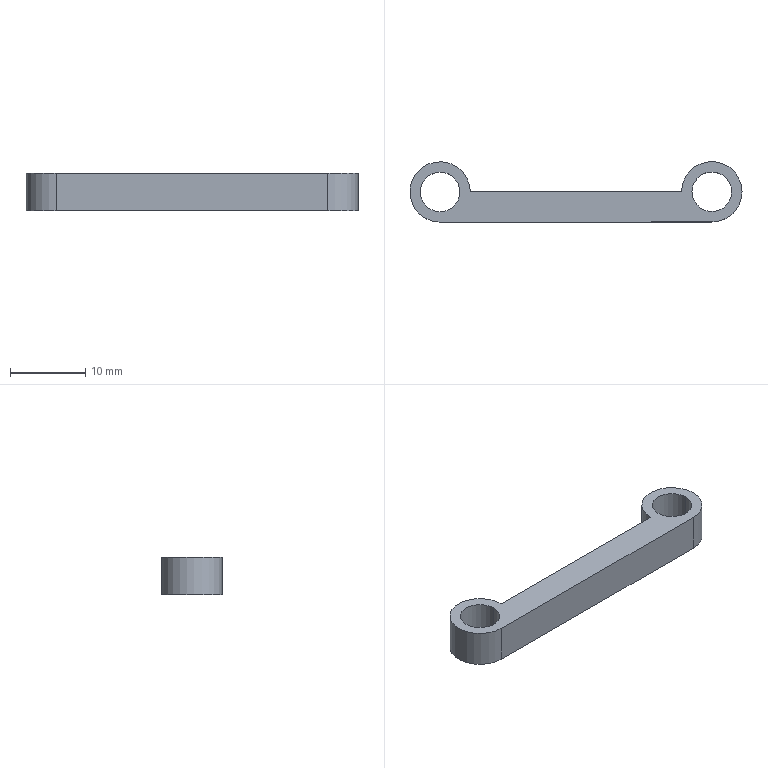Part | SolidWorks | features ICE 10, Fillet 4, Attribute 1, Extrusion 1 | 1 solid | 11 faces | box 44 x 8.023 x 5 mm | volume 880.516 mm3 | cylinder 7 | plane 4 | commonest cylinder face diameters 5.25 x4 8 x3
STEP:
#1=CARTESIAN_POINT('',(-13.375,0.,0.));
#2=VERTEX_POINT('',#1);
#3=CARTESIAN_POINT('',(-18.625,0.,0.));
#4=VERTEX_POINT('',#3);
#5=CARTESIAN_POINT('',(-16.,0.,0.));
#6=DIRECTION('',(0.,0.,-1.));
#7=DIRECTION('',(-1.,0.,0.));
#8=AXIS2_PLACEMENT_3D('',#5,#6,#7);
#9=CIRCLE('',#8,2.625);
#10=EDGE_CURVE('',#2,#4,#9,.T.);
#11=ORIENTED_EDGE('',*,*,#10,.T.);
#12=CARTESIAN_POINT('',(-18.625,0.,5.));
#13=VERTEX_POINT('',#12);
#14=CARTESIAN_POINT('',(-18.625,0.,-20.));
#15=DIRECTION('',(0.,0.,1.));
#16=VECTOR('',#15,1000.);
#17=LINE('',#14,#16);
#18=EDGE_CURVE('',#4,#13,#17,.T.);
#19=ORIENTED_EDGE('',*,*,#18,.T.);
#20=CARTESIAN_POINT('',(-13.375,0.,5.));
#21=VERTEX_POINT('',#20);
#22=CARTESIAN_POINT('',(-16.,0.,5.));
#23=DIRECTION('',(0.,0.,-1.));
#24=DIRECTION('',(-1.,0.,0.));
#25=AXIS2_PLACEMENT_3D('',#22,#23,#24);
#26=CIRCLE('',#25,2.625);
#27=EDGE_CURVE('',#21,#13,#26,.T.);
#28=ORIENTED_EDGE('',*,*,#27,.F.);
#29=CARTESIAN_POINT('',(-13.375,0.,-20.));
#30=DIRECTION('',(0.,0.,1.));
#31=VECTOR('',#30,1000.);
#32=LINE('',#29,#31);
#33=EDGE_CURVE('',#2,#21,#32,.T.);
#34=ORIENTED_EDGE('',*,*,#33,.F.);
#35=EDGE_LOOP('',(#11,#19,#28,#34));
#36=FACE_OUTER_BOUND('',#35,.T.);
#37=CARTESIAN_POINT('',(-16.,0.,-20.));
#38=DIRECTION('',(0.,0.,1.));
#39=DIRECTION('',(1.,0.,0.));
#40=AXIS2_PLACEMENT_3D('',#37,#38,#39);
#41=CYLINDRICAL_SURFACE('',#40,2.625);
#42=ADVANCED_FACE('',(#36),#41,.F.);
#43=CARTESIAN_POINT('',(17.375,0.02311,0.));
#44=VERTEX_POINT('',#43);
#45=CARTESIAN_POINT('',(22.625,0.02311,0.));
#46=VERTEX_POINT('',#45);
#47=CARTESIAN_POINT('',(20.,0.02311,0.));
#48=DIRECTION('',(0.,0.,1.));
#49=DIRECTION('',(1.,0.,0.));
#50=AXIS2_PLACEMENT_3D('',#47,#48,#49);
#51=CIRCLE('',#50,2.625);
#52=EDGE_CURVE('',#44,#46,#51,.T.);
#53=ORIENTED_EDGE('',*,*,#52,.F.);
#54=CARTESIAN_POINT('',(17.375,0.02311,5.));
#55=VERTEX_POINT('',#54);
#56=CARTESIAN_POINT('',(17.375,0.02311,0.));
#57=DIRECTION('',(0.,0.,1.));
#58=VECTOR('',#57,1000.);
#59=LINE('',#56,#58);
#60=EDGE_CURVE('',#44,#55,#59,.T.);
#61=ORIENTED_EDGE('',*,*,#60,.T.);
#62=CARTESIAN_POINT('',(22.625,0.02311,5.));
#63=VERTEX_POINT('',#62);
#64=CARTESIAN_POINT('',(20.,0.02311,5.));
#65=DIRECTION('',(0.,0.,1.));
#66=DIRECTION('',(1.,0.,0.));
#67=AXIS2_PLACEMENT_3D('',#64,#65,#66);
#68=CIRCLE('',#67,2.625);
#69=EDGE_CURVE('',#55,#63,#68,.T.);
#70=ORIENTED_EDGE('',*,*,#69,.T.);
#71=CARTESIAN_POINT('',(22.625,0.02311,0.));
#72=DIRECTION('',(0.,0.,1.));
#73=VECTOR('',#72,1000.);
#74=LINE('',#71,#73);
#75=EDGE_CURVE('',#46,#63,#74,.T.);
#76=ORIENTED_EDGE('',*,*,#75,.F.);
#77=EDGE_LOOP('',(#53,#61,#70,#76));
#78=FACE_OUTER_BOUND('',#77,.T.);
#79=CARTESIAN_POINT('',(20.,0.02311,0.));
#80=DIRECTION('',(0.,0.,1.));
#81=DIRECTION('',(1.,0.,0.));
#82=AXIS2_PLACEMENT_3D('',#79,#80,#81);
#83=CYLINDRICAL_SURFACE('',#82,2.625);
#84=ADVANCED_FACE('',(#78),#83,.F.);
#85=CARTESIAN_POINT('',(20.,-3.977,0.));
#86=VERTEX_POINT('',#85);
#87=CARTESIAN_POINT('',(24.,0.02311,0.));
#88=VERTEX_POINT('',#87);
#89=CARTESIAN_POINT('',(20.,0.02311,0.));
#90=DIRECTION('',(0.,0.,1.));
#91=DIRECTION('',(1.,0.,0.));
#92=AXIS2_PLACEMENT_3D('',#89,#90,#91);
#93=CIRCLE('',#92,4.);
#94=EDGE_CURVE('',#86,#88,#93,.T.);
#95=ORIENTED_EDGE('',*,*,#94,.T.);
#96=CARTESIAN_POINT('',(24.,0.02311,5.));
#97=VERTEX_POINT('',#96);
#98=CARTESIAN_POINT('',(24.,0.02311,0.));
#99=DIRECTION('',(0.,0.,1.));
#100=VECTOR('',#99,1000.);
#101=LINE('',#98,#100);
#102=EDGE_CURVE('',#88,#97,#101,.T.);
#103=ORIENTED_EDGE('',*,*,#102,.T.);
#104=CARTESIAN_POINT('',(20.,-3.977,5.));
#105=VERTEX_POINT('',#104);
#106=CARTESIAN_POINT('',(20.,0.02311,5.));
#107=DIRECTION('',(0.,0.,1.));
#108=DIRECTION('',(1.,0.,0.));
#109=AXIS2_PLACEMENT_3D('',#106,#107,#108);
#110=CIRCLE('',#109,4.);
#111=EDGE_CURVE('',#105,#97,#110,.T.);
#112=ORIENTED_EDGE('',*,*,#111,.F.);
#113=CARTESIAN_POINT('',(20.,-3.977,0.));
#114=DIRECTION('',(0.,0.,1.));
#115=VECTOR('',#114,1000.);
#116=LINE('',#113,#115);
#117=EDGE_CURVE('',#86,#105,#116,.T.);
#118=ORIENTED_EDGE('',*,*,#117,.F.);
#119=EDGE_LOOP('',(#95,#103,#112,#118));
#120=FACE_OUTER_BOUND('',#119,.T.);
#121=CARTESIAN_POINT('',(20.,0.02311,0.));
#122=DIRECTION('',(0.,0.,1.));
#123=DIRECTION('',(1.,0.,0.));
#124=AXIS2_PLACEMENT_3D('',#121,#122,#123);
#125=CYLINDRICAL_SURFACE('',#124,4.);
#126=ADVANCED_FACE('',(#120),#125,.T.);
#127=ORIENTED_EDGE('',*,*,#27,.T.);
#128=CARTESIAN_POINT('',(-16.,0.,5.));
#129=DIRECTION('',(0.,0.,-1.));
#130=DIRECTION('',(-1.,0.,0.));
#131=AXIS2_PLACEMENT_3D('',#128,#129,#130);
#132=CIRCLE('',#131,2.625);
#133=EDGE_CURVE('',#13,#21,#132,.T.);
#134=ORIENTED_EDGE('',*,*,#133,.T.);
#135=EDGE_LOOP('',(#127,#134));
#136=FACE_BOUND('',#135,.T.);
#137=CARTESIAN_POINT('',(-12.,0.,5.));
#138=VERTEX_POINT('',#137);
#139=CARTESIAN_POINT('',(-15.997,-4.,5.));
#140=VERTEX_POINT('',#139);
#141=CARTESIAN_POINT('',(-16.,0.,5.));
#142=DIRECTION('',(0.,0.,1.));
#143=DIRECTION('',(1.,0.,0.));
#144=AXIS2_PLACEMENT_3D('',#141,#142,#143);
#145=CIRCLE('',#144,4.);
#146=EDGE_CURVE('',#138,#140,#145,.T.);
#147=ORIENTED_EDGE('',*,*,#146,.T.);
#148=CARTESIAN_POINT('',(-16.,-4.,5.));
#149=DIRECTION('',(1.,0.0006418,0.));
#150=VECTOR('',#149,1000.);
#151=LINE('',#148,#150);
#152=EDGE_CURVE('',#140,#105,#151,.T.);
#153=ORIENTED_EDGE('',*,*,#152,.T.);
#154=ORIENTED_EDGE('',*,*,#111,.T.);
#155=CARTESIAN_POINT('',(16.,0.02311,5.));
#156=VERTEX_POINT('',#155);
#157=CARTESIAN_POINT('',(20.,0.02311,5.));
#158=DIRECTION('',(0.,0.,1.));
#159=DIRECTION('',(1.,0.,0.));
#160=AXIS2_PLACEMENT_3D('',#157,#158,#159);
#161=CIRCLE('',#160,4.);
#162=EDGE_CURVE('',#97,#156,#161,.T.);
#163=ORIENTED_EDGE('',*,*,#162,.T.);
#164=CARTESIAN_POINT('',(-12.,0.,5.));
#165=DIRECTION('',(1.,0.0008252,0.));
#166=VECTOR('',#165,1000.);
#167=LINE('',#164,#166);
#168=EDGE_CURVE('',#138,#156,#167,.T.);
#169=ORIENTED_EDGE('',*,*,#168,.F.);
#170=EDGE_LOOP('',(#147,#153,#154,#163,#169));
#171=FACE_OUTER_BOUND('',#170,.T.);
#172=CARTESIAN_POINT('',(20.,0.02311,5.));
#173=DIRECTION('',(0.,0.,1.));
#174=DIRECTION('',(1.,0.,0.));
#175=AXIS2_PLACEMENT_3D('',#172,#173,#174);
#176=CIRCLE('',#175,2.625);
#177=EDGE_CURVE('',#63,#55,#176,.T.);
#178=ORIENTED_EDGE('',*,*,#177,.F.);
#179=ORIENTED_EDGE('',*,*,#69,.F.);
#180=EDGE_LOOP('',(#178,#179));
#181=FACE_BOUND('',#180,.T.);
#182=CARTESIAN_POINT('',(0.,0.,5.));
#183=DIRECTION('',(0.,0.,-1.));
#184=DIRECTION('',(-1.,0.,0.));
#185=AXIS2_PLACEMENT_3D('',#182,#183,#184);
#186=PLANE('',#185);
#187=ADVANCED_FACE('',(#136,#171,#181),#186,.F.);
#188=CARTESIAN_POINT('',(-15.997,-4.,0.));
#189=VERTEX_POINT('',#188);
#190=CARTESIAN_POINT('',(-16.,-4.,0.));
#191=DIRECTION('',(1.,0.0006418,0.));
#192=VECTOR('',#191,1000.);
#193=LINE('',#190,#192);
#194=EDGE_CURVE('',#189,#86,#193,.T.);
#195=ORIENTED_EDGE('',*,*,#194,.F.);
#196=CARTESIAN_POINT('',(-12.,0.,0.));
#197=VERTEX_POINT('',#196);
#198=CARTESIAN_POINT('',(-16.,0.,0.));
#199=DIRECTION('',(0.,0.,1.));
#200=DIRECTION('',(1.,0.,0.));
#201=AXIS2_PLACEMENT_3D('',#198,#199,#200);
#202=CIRCLE('',#201,4.);
#203=EDGE_CURVE('',#197,#189,#202,.T.);
#204=ORIENTED_EDGE('',*,*,#203,.F.);
#205=CARTESIAN_POINT('',(16.,0.02311,0.));
#206=VERTEX_POINT('',#205);
#207=CARTESIAN_POINT('',(-12.,0.,0.));
#208=DIRECTION('',(1.,0.0008252,0.));
#209=VECTOR('',#208,1000.);
#210=LINE('',#207,#209);
#211=EDGE_CURVE('',#197,#206,#210,.T.);
#212=ORIENTED_EDGE('',*,*,#211,.T.);
#213=CARTESIAN_POINT('',(20.,0.02311,0.));
#214=DIRECTION('',(0.,0.,1.));
#215=DIRECTION('',(1.,0.,0.));
#216=AXIS2_PLACEMENT_3D('',#213,#214,#215);
#217=CIRCLE('',#216,4.);
#218=EDGE_CURVE('',#88,#206,#217,.T.);
#219=ORIENTED_EDGE('',*,*,#218,.F.);
#220=ORIENTED_EDGE('',*,*,#94,.F.);
#221=EDGE_LOOP('',(#195,#204,#212,#219,#220));
#222=FACE_OUTER_BOUND('',#221,.T.);
#223=ORIENTED_EDGE('',*,*,#10,.F.);
#224=CARTESIAN_POINT('',(-16.,0.,0.));
#225=DIRECTION('',(0.,0.,-1.));
#226=DIRECTION('',(-1.,0.,0.));
#227=AXIS2_PLACEMENT_3D('',#224,#225,#226);
#228=CIRCLE('',#227,2.625);
#229=EDGE_CURVE('',#4,#2,#228,.T.);
#230=ORIENTED_EDGE('',*,*,#229,.F.);
#231=EDGE_LOOP('',(#223,#230));
#232=FACE_BOUND('',#231,.T.);
#233=CARTESIAN_POINT('',(20.,0.02311,0.));
#234=DIRECTION('',(0.,0.,1.));
#235=DIRECTION('',(1.,0.,0.));
#236=AXIS2_PLACEMENT_3D('',#233,#234,#235);
#237=CIRCLE('',#236,2.625);
#238=EDGE_CURVE('',#46,#44,#237,.T.);
#239=ORIENTED_EDGE('',*,*,#238,.T.);
#240=ORIENTED_EDGE('',*,*,#52,.T.);
#241=EDGE_LOOP('',(#239,#240));
#242=FACE_BOUND('',#241,.T.);
#243=CARTESIAN_POINT('',(0.,0.,0.));
#244=DIRECTION('',(0.,0.,-1.));
#245=DIRECTION('',(-1.,0.,0.));
#246=AXIS2_PLACEMENT_3D('',#243,#244,#245);
#247=PLANE('',#246);
#248=ADVANCED_FACE('',(#222,#232,#242),#247,.T.);
#249=ORIENTED_EDGE('',*,*,#102,.F.);
#250=ORIENTED_EDGE('',*,*,#218,.T.);
#251=CARTESIAN_POINT('',(16.,0.02311,0.));
#252=DIRECTION('',(0.,0.,1.));
#253=VECTOR('',#252,1000.);
#254=LINE('',#251,#253);
#255=EDGE_CURVE('',#206,#156,#254,.T.);
#256=ORIENTED_EDGE('',*,*,#255,.T.);
#257=ORIENTED_EDGE('',*,*,#162,.F.);
#258=EDGE_LOOP('',(#249,#250,#256,#257));
#259=FACE_OUTER_BOUND('',#258,.T.);
#260=CARTESIAN_POINT('',(20.,0.02311,0.));
#261=DIRECTION('',(0.,0.,1.));
#262=DIRECTION('',(1.,0.,0.));
#263=AXIS2_PLACEMENT_3D('',#260,#261,#262);
#264=CYLINDRICAL_SURFACE('',#263,4.);
#265=ADVANCED_FACE('',(#259),#264,.T.);
#266=ORIENTED_EDGE('',*,*,#60,.F.);
#267=ORIENTED_EDGE('',*,*,#238,.F.);
#268=ORIENTED_EDGE('',*,*,#75,.T.);
#269=ORIENTED_EDGE('',*,*,#177,.T.);
#270=EDGE_LOOP('',(#266,#267,#268,#269));
#271=FACE_OUTER_BOUND('',#270,.T.);
#272=CARTESIAN_POINT('',(20.,0.02311,0.));
#273=DIRECTION('',(0.,0.,1.));
#274=DIRECTION('',(1.,0.,0.));
#275=AXIS2_PLACEMENT_3D('',#272,#273,#274);
#276=CYLINDRICAL_SURFACE('',#275,2.625);
#277=ADVANCED_FACE('',(#271),#276,.F.);
#278=ORIENTED_EDGE('',*,*,#203,.T.);
#279=CARTESIAN_POINT('',(-15.997,-4.,0.));
#280=DIRECTION('',(0.,0.,-1.));
#281=VECTOR('',#280,1000.);
#282=LINE('',#279,#281);
#283=EDGE_CURVE('',#140,#189,#282,.T.);
#284=ORIENTED_EDGE('',*,*,#283,.F.);
#285=ORIENTED_EDGE('',*,*,#146,.F.);
#286=CARTESIAN_POINT('',(-12.,0.,0.));
#287=DIRECTION('',(0.,0.,1.));
#288=VECTOR('',#287,1000.);
#289=LINE('',#286,#288);
#290=EDGE_CURVE('',#197,#138,#289,.T.);
#291=ORIENTED_EDGE('',*,*,#290,.F.);
#292=EDGE_LOOP('',(#278,#284,#285,#291));
#293=FACE_OUTER_BOUND('',#292,.T.);
#294=CARTESIAN_POINT('',(-16.,0.,0.));
#295=DIRECTION('',(0.,0.,1.));
#296=DIRECTION('',(1.,0.,0.));
#297=AXIS2_PLACEMENT_3D('',#294,#295,#296);
#298=CYLINDRICAL_SURFACE('',#297,4.);
#299=ADVANCED_FACE('',(#293),#298,.T.);
#300=ORIENTED_EDGE('',*,*,#18,.F.);
#301=ORIENTED_EDGE('',*,*,#229,.T.);
#302=ORIENTED_EDGE('',*,*,#33,.T.);
#303=ORIENTED_EDGE('',*,*,#133,.F.);
#304=EDGE_LOOP('',(#300,#301,#302,#303));
#305=FACE_OUTER_BOUND('',#304,.T.);
#306=CARTESIAN_POINT('',(-16.,0.,-20.));
#307=DIRECTION('',(0.,0.,1.));
#308=DIRECTION('',(1.,0.,0.));
#309=AXIS2_PLACEMENT_3D('',#306,#307,#308);
#310=CYLINDRICAL_SURFACE('',#309,2.625);
#311=ADVANCED_FACE('',(#305),#310,.F.);
#312=ORIENTED_EDGE('',*,*,#168,.T.);
#313=ORIENTED_EDGE('',*,*,#255,.F.);
#314=ORIENTED_EDGE('',*,*,#211,.F.);
#315=ORIENTED_EDGE('',*,*,#290,.T.);
#316=EDGE_LOOP('',(#312,#313,#314,#315));
#317=FACE_OUTER_BOUND('',#316,.T.);
#318=CARTESIAN_POINT('',(-12.,0.,0.));
#319=DIRECTION('',(0.0008252,-1.,0.));
#320=DIRECTION('',(1.,0.0008252,0.));
#321=AXIS2_PLACEMENT_3D('',#318,#319,#320);
#322=PLANE('',#321);
#323=ADVANCED_FACE('',(#317),#322,.F.);
#324=ORIENTED_EDGE('',*,*,#152,.F.);
#325=ORIENTED_EDGE('',*,*,#283,.T.);
#326=ORIENTED_EDGE('',*,*,#194,.T.);
#327=ORIENTED_EDGE('',*,*,#117,.T.);
#328=EDGE_LOOP('',(#324,#325,#326,#327));
#329=FACE_OUTER_BOUND('',#328,.T.);
#330=CARTESIAN_POINT('',(-16.,-4.,0.));
#331=DIRECTION('',(0.0006418,-1.,0.));
#332=DIRECTION('',(1.,0.0006418,0.));
#333=AXIS2_PLACEMENT_3D('',#330,#331,#332);
#334=PLANE('',#333);
#335=ADVANCED_FACE('',(#329),#334,.T.);
#336=CLOSED_SHELL('',(#42,#84,#126,#187,#248,#265,#277,#299,#311,#323,#335));
#337=MANIFOLD_SOLID_BREP('',#336);
#338=CARTESIAN_POINT('',(0.,0.,0.));
#339=DIRECTION('',(0.,0.,1.));
#340=DIRECTION('',(1.,0.,0.));
#341=AXIS2_PLACEMENT_3D('',#338,#339,#340);
#342=(LENGTH_UNIT()NAMED_UNIT(*)SI_UNIT(.MILLI.,.METRE.));
#343=UNCERTAINTY_MEASURE_WITH_UNIT(LENGTH_MEASURE(0.00001),#342,'','');
#344=(NAMED_UNIT(*)PLANE_ANGLE_UNIT()SI_UNIT($,.RADIAN.));
#345=(NAMED_UNIT(*)SI_UNIT($,.STERADIAN.)SOLID_ANGLE_UNIT());
#346=(GEOMETRIC_REPRESENTATION_CONTEXT(3)GLOBAL_UNCERTAINTY_ASSIGNED_CONTEXT((#343))GLOBAL_UNIT_ASSIGNED_CONTEXT((#342,#344,#345))REPRESENTATION_CONTEXT('',''));
#347=ADVANCED_BREP_SHAPE_REPRESENTATION('',(#337,#341),#346);